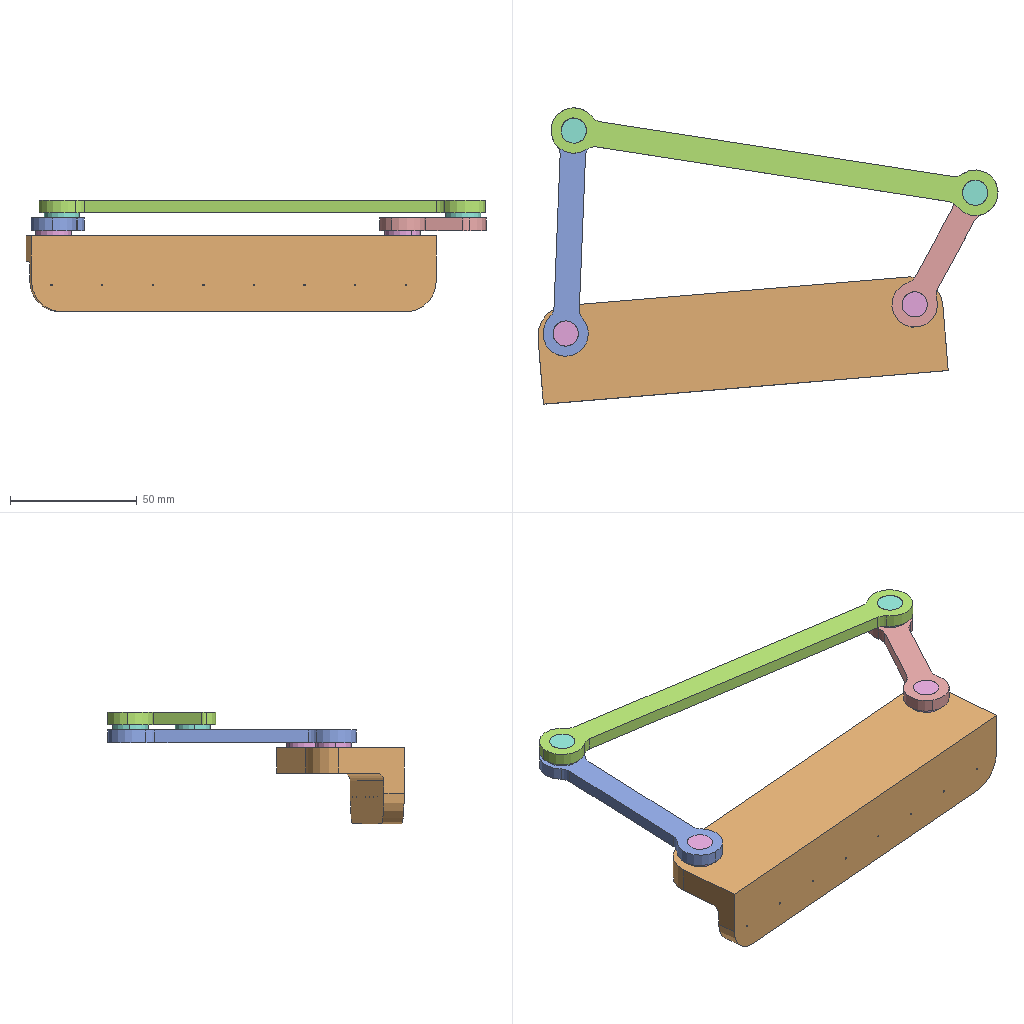Assembly | SolidWorks | 6 different items | 8 placed | box 181 x 117 x 44 mm
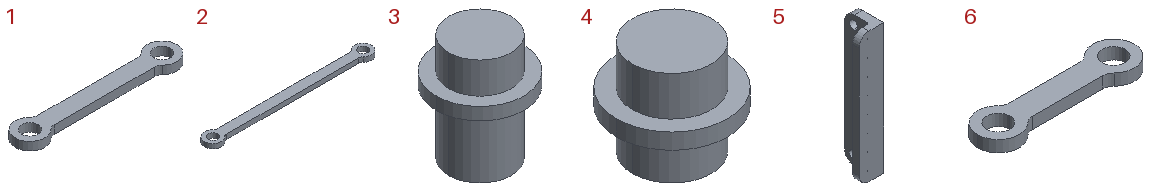Parts list (item | quantity | size | volume | features):
1 | x1 | 98 x 18 x 5 mm | 4921 mm3 | features Extrusion 1
2 | x1 | 178 x 18 x 5 mm | 8921 mm3 | features Extrusion 1
3 | x2 | 14 x 14 x 17 mm | 1486 mm3 | features ICE 2, Extrusion 1
4 | x2 | 14 x 14 x 12 mm | 1093 mm3 | features ICE 2, Extrusion 1
5 | x1 | 30 x 38 x 160 mm | 83802 mm3 | features ICE 3, Fillet 2, Extrusion 1
6 | x1 | 68 x 18 x 5 mm | 3421 mm3 | features Extrusion 1
Mates (type | each side: item.copy, entity, surface, feature):
Concentric | 3.1 face cylinder Boss-Extrude1 | 5.1 face cylinder Cut-Extrude1
Concentric | 6.1 face cylinder Boss-Extrude1 | 3.1 face cylinder Boss-Extrude3
Coincident | 3.1 face plane Boss-Extrude2 | 5.1 face plane Boss-Extrude1
Coincident | 6.1 face plane Boss-Extrude1 | 3.1 face plane Boss-Extrude2
Concentric | 6.1 face cylinder Boss-Extrude1 | 4.1 face cylinder Boss-Extrude1
Coincident | 6.1 face plane Boss-Extrude1 | 4.1 face plane Boss-Extrude2
Concentric | 2.1 face cylinder Boss-Extrude1 | 4.1 face cylinder Boss-Extrude3
Coincident | 2.1 face plane Boss-Extrude1 | 4.1 face plane Boss-Extrude2
Concentric | 5.1 face cylinder Cut-Extrude1 | 3.2 face cylinder Boss-Extrude1
Coincident | 5.1 face plane Boss-Extrude1 | 3.2 face plane Boss-Extrude2
Concentric | 1.1 face cylinder Boss-Extrude1 | 3.2 face cylinder Boss-Extrude3
Coincident | 1.1 face plane Boss-Extrude1 | 3.2 face plane Boss-Extrude2
Concentric | 1.1 face cylinder Boss-Extrude1 | 4.2 face cylinder Boss-Extrude1
Coincident | 1.1 face plane Boss-Extrude1 | 4.2 face plane Boss-Extrude2
Concentric | 2.1 face cylinder Boss-Extrude1 | 4.2 face cylinder Boss-Extrude3